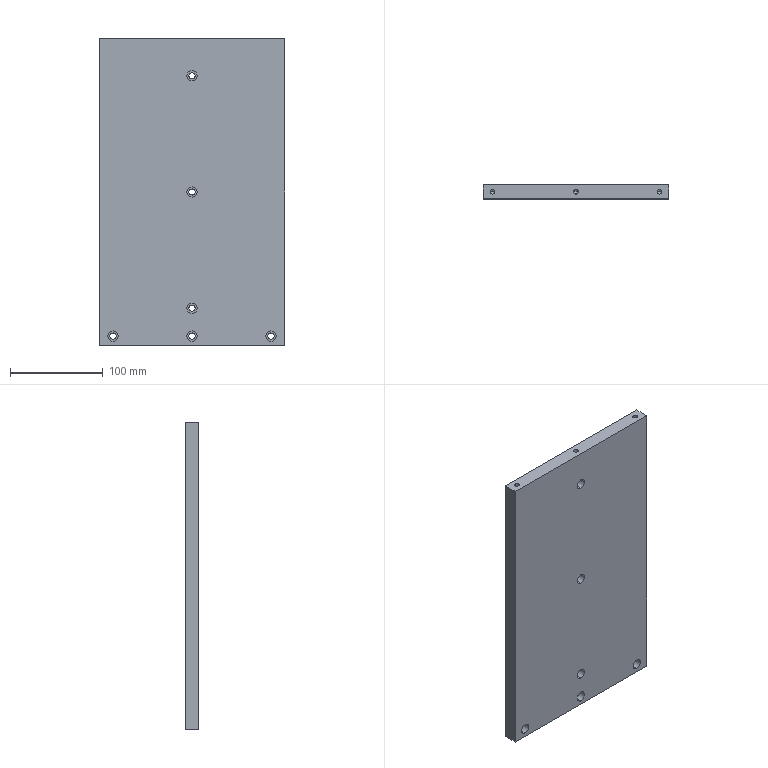Part | SolidWorks | features HoleWzd 3, Extrusion 1 | 1 solid | 48 faces | box 200 x 15 x 330 mm | volume 982971 mm3 | cylinder 30 | plane 12 | cone 6 | commonest cylinder face diameters 6.6 x12 11 x12 5 x6
STEP:
#1=CARTESIAN_POINT('',(-2.5,0.,148.));
#2=VERTEX_POINT('',#1);
#3=CARTESIAN_POINT('',(2.5,0.,148.));
#4=VERTEX_POINT('',#3);
#5=CARTESIAN_POINT('',(0.,0.,148.));
#6=DIRECTION('',(0.,0.,1.));
#7=DIRECTION('',(1.,0.,0.));
#8=AXIS2_PLACEMENT_3D('',#5,#6,#7);
#9=CIRCLE('',#8,2.5);
#10=EDGE_CURVE('',#2,#4,#9,.T.);
#11=ORIENTED_EDGE('',*,*,#10,.F.);
#12=CARTESIAN_POINT('',(-2.5,0.,165.));
#13=VERTEX_POINT('',#12);
#14=CARTESIAN_POINT('',(-2.5,0.,165.));
#15=DIRECTION('',(0.,0.,1.));
#16=VECTOR('',#15,1000.);
#17=LINE('',#14,#16);
#18=EDGE_CURVE('',#2,#13,#17,.T.);
#19=ORIENTED_EDGE('',*,*,#18,.T.);
#20=CARTESIAN_POINT('',(2.5,0.,165.));
#21=VERTEX_POINT('',#20);
#22=CARTESIAN_POINT('',(0.,0.,165.));
#23=DIRECTION('',(0.,0.,1.));
#24=DIRECTION('',(1.,0.,0.));
#25=AXIS2_PLACEMENT_3D('',#22,#23,#24);
#26=CIRCLE('',#25,2.5);
#27=EDGE_CURVE('',#13,#21,#26,.T.);
#28=ORIENTED_EDGE('',*,*,#27,.T.);
#29=CARTESIAN_POINT('',(2.5,0.,165.));
#30=DIRECTION('',(0.,0.,1.));
#31=VECTOR('',#30,1000.);
#32=LINE('',#29,#31);
#33=EDGE_CURVE('',#4,#21,#32,.T.);
#34=ORIENTED_EDGE('',*,*,#33,.F.);
#35=EDGE_LOOP('',(#11,#19,#28,#34));
#36=FACE_OUTER_BOUND('',#35,.T.);
#37=CARTESIAN_POINT('',(0.,0.,165.));
#38=DIRECTION('',(0.,0.,1.));
#39=DIRECTION('',(1.,0.,0.));
#40=AXIS2_PLACEMENT_3D('',#37,#38,#39);
#41=CYLINDRICAL_SURFACE('',#40,2.5);
#42=ADVANCED_FACE('',(#36),#41,.F.);
#43=CARTESIAN_POINT('',(0.,0.,146.498));
#44=VERTEX_POINT('',#43);
#45=CARTESIAN_POINT('',(2.5,0.,148.));
#46=DIRECTION('',(0.8572,0.,0.515));
#47=VECTOR('',#46,1000.);
#48=LINE('',#45,#47);
#49=EDGE_CURVE('',#44,#4,#48,.T.);
#50=ORIENTED_EDGE('',*,*,#49,.F.);
#51=CARTESIAN_POINT('',(-2.5,0.,148.));
#52=DIRECTION('',(-0.8572,0.,0.515));
#53=VECTOR('',#52,1000.);
#54=LINE('',#51,#53);
#55=EDGE_CURVE('',#44,#2,#54,.T.);
#56=ORIENTED_EDGE('',*,*,#55,.T.);
#57=ORIENTED_EDGE('',*,*,#10,.T.);
#58=EDGE_LOOP('',(#50,#56,#57));
#59=FACE_OUTER_BOUND('',#58,.T.);
#60=CARTESIAN_POINT('',(0.,0.,148.));
#61=DIRECTION('',(0.,0.,1.));
#62=DIRECTION('',(1.,0.,0.));
#63=AXIS2_PLACEMENT_3D('',#60,#61,#62);
#64=CONICAL_SURFACE('',#63,2.5,1.03);
#65=ADVANCED_FACE('',(#59),#64,.F.);
#66=CARTESIAN_POINT('',(-92.5,0.,148.));
#67=VERTEX_POINT('',#66);
#68=CARTESIAN_POINT('',(-87.5,0.,148.));
#69=VERTEX_POINT('',#68);
#70=CARTESIAN_POINT('',(-90.,0.,148.));
#71=DIRECTION('',(0.,0.,1.));
#72=DIRECTION('',(1.,0.,0.));
#73=AXIS2_PLACEMENT_3D('',#70,#71,#72);
#74=CIRCLE('',#73,2.5);
#75=EDGE_CURVE('',#67,#69,#74,.T.);
#76=ORIENTED_EDGE('',*,*,#75,.F.);
#77=CARTESIAN_POINT('',(-92.5,0.,165.));
#78=VERTEX_POINT('',#77);
#79=CARTESIAN_POINT('',(-92.5,0.,165.));
#80=DIRECTION('',(0.,0.,1.));
#81=VECTOR('',#80,1000.);
#82=LINE('',#79,#81);
#83=EDGE_CURVE('',#67,#78,#82,.T.);
#84=ORIENTED_EDGE('',*,*,#83,.T.);
#85=CARTESIAN_POINT('',(-87.5,0.,165.));
#86=VERTEX_POINT('',#85);
#87=CARTESIAN_POINT('',(-90.,0.,165.));
#88=DIRECTION('',(0.,0.,1.));
#89=DIRECTION('',(1.,0.,0.));
#90=AXIS2_PLACEMENT_3D('',#87,#88,#89);
#91=CIRCLE('',#90,2.5);
#92=EDGE_CURVE('',#78,#86,#91,.T.);
#93=ORIENTED_EDGE('',*,*,#92,.T.);
#94=CARTESIAN_POINT('',(-87.5,0.,165.));
#95=DIRECTION('',(0.,0.,1.));
#96=VECTOR('',#95,1000.);
#97=LINE('',#94,#96);
#98=EDGE_CURVE('',#69,#86,#97,.T.);
#99=ORIENTED_EDGE('',*,*,#98,.F.);
#100=EDGE_LOOP('',(#76,#84,#93,#99));
#101=FACE_OUTER_BOUND('',#100,.T.);
#102=CARTESIAN_POINT('',(-90.,0.,165.));
#103=DIRECTION('',(0.,0.,1.));
#104=DIRECTION('',(1.,0.,0.));
#105=AXIS2_PLACEMENT_3D('',#102,#103,#104);
#106=CYLINDRICAL_SURFACE('',#105,2.5);
#107=ADVANCED_FACE('',(#101),#106,.F.);
#108=CARTESIAN_POINT('',(-90.,0.,146.498));
#109=VERTEX_POINT('',#108);
#110=CARTESIAN_POINT('',(-87.5,0.,148.));
#111=DIRECTION('',(0.8572,0.,0.515));
#112=VECTOR('',#111,1000.);
#113=LINE('',#110,#112);
#114=EDGE_CURVE('',#109,#69,#113,.T.);
#115=ORIENTED_EDGE('',*,*,#114,.F.);
#116=CARTESIAN_POINT('',(-92.5,0.,148.));
#117=DIRECTION('',(-0.8572,0.,0.515));
#118=VECTOR('',#117,1000.);
#119=LINE('',#116,#118);
#120=EDGE_CURVE('',#109,#67,#119,.T.);
#121=ORIENTED_EDGE('',*,*,#120,.T.);
#122=ORIENTED_EDGE('',*,*,#75,.T.);
#123=EDGE_LOOP('',(#115,#121,#122));
#124=FACE_OUTER_BOUND('',#123,.T.);
#125=CARTESIAN_POINT('',(-90.,0.,148.));
#126=DIRECTION('',(0.,0.,1.));
#127=DIRECTION('',(1.,0.,0.));
#128=AXIS2_PLACEMENT_3D('',#125,#126,#127);
#129=CONICAL_SURFACE('',#128,2.5,1.03);
#130=ADVANCED_FACE('',(#124),#129,.F.);
#131=CARTESIAN_POINT('',(87.5,0.,148.));
#132=VERTEX_POINT('',#131);
#133=CARTESIAN_POINT('',(92.5,0.,148.));
#134=VERTEX_POINT('',#133);
#135=CARTESIAN_POINT('',(90.,0.,148.));
#136=DIRECTION('',(0.,0.,1.));
#137=DIRECTION('',(1.,0.,0.));
#138=AXIS2_PLACEMENT_3D('',#135,#136,#137);
#139=CIRCLE('',#138,2.5);
#140=EDGE_CURVE('',#132,#134,#139,.T.);
#141=ORIENTED_EDGE('',*,*,#140,.F.);
#142=CARTESIAN_POINT('',(87.5,0.,165.));
#143=VERTEX_POINT('',#142);
#144=CARTESIAN_POINT('',(87.5,0.,165.));
#145=DIRECTION('',(0.,0.,1.));
#146=VECTOR('',#145,1000.);
#147=LINE('',#144,#146);
#148=EDGE_CURVE('',#132,#143,#147,.T.);
#149=ORIENTED_EDGE('',*,*,#148,.T.);
#150=CARTESIAN_POINT('',(92.5,0.,165.));
#151=VERTEX_POINT('',#150);
#152=CARTESIAN_POINT('',(90.,0.,165.));
#153=DIRECTION('',(0.,0.,1.));
#154=DIRECTION('',(1.,0.,0.));
#155=AXIS2_PLACEMENT_3D('',#152,#153,#154);
#156=CIRCLE('',#155,2.5);
#157=EDGE_CURVE('',#143,#151,#156,.T.);
#158=ORIENTED_EDGE('',*,*,#157,.T.);
#159=CARTESIAN_POINT('',(92.5,0.,165.));
#160=DIRECTION('',(0.,0.,1.));
#161=VECTOR('',#160,1000.);
#162=LINE('',#159,#161);
#163=EDGE_CURVE('',#134,#151,#162,.T.);
#164=ORIENTED_EDGE('',*,*,#163,.F.);
#165=EDGE_LOOP('',(#141,#149,#158,#164));
#166=FACE_OUTER_BOUND('',#165,.T.);
#167=CARTESIAN_POINT('',(90.,0.,165.));
#168=DIRECTION('',(0.,0.,1.));
#169=DIRECTION('',(1.,0.,0.));
#170=AXIS2_PLACEMENT_3D('',#167,#168,#169);
#171=CYLINDRICAL_SURFACE('',#170,2.5);
#172=ADVANCED_FACE('',(#166),#171,.F.);
#173=CARTESIAN_POINT('',(90.,0.,146.498));
#174=VERTEX_POINT('',#173);
#175=CARTESIAN_POINT('',(92.5,0.,148.));
#176=DIRECTION('',(0.8572,0.,0.515));
#177=VECTOR('',#176,1000.);
#178=LINE('',#175,#177);
#179=EDGE_CURVE('',#174,#134,#178,.T.);
#180=ORIENTED_EDGE('',*,*,#179,.F.);
#181=CARTESIAN_POINT('',(87.5,0.,148.));
#182=DIRECTION('',(-0.8572,0.,0.515));
#183=VECTOR('',#182,1000.);
#184=LINE('',#181,#183);
#185=EDGE_CURVE('',#174,#132,#184,.T.);
#186=ORIENTED_EDGE('',*,*,#185,.T.);
#187=ORIENTED_EDGE('',*,*,#140,.T.);
#188=EDGE_LOOP('',(#180,#186,#187));
#189=FACE_OUTER_BOUND('',#188,.T.);
#190=CARTESIAN_POINT('',(90.,0.,148.));
#191=DIRECTION('',(0.,0.,1.));
#192=DIRECTION('',(1.,0.,0.));
#193=AXIS2_PLACEMENT_3D('',#190,#191,#192);
#194=CONICAL_SURFACE('',#193,2.5,1.03);
#195=ADVANCED_FACE('',(#189),#194,.F.);
#196=CARTESIAN_POINT('',(-85.,0.5,-149.5));
#197=VERTEX_POINT('',#196);
#198=CARTESIAN_POINT('',(-85.,0.5,-160.5));
#199=VERTEX_POINT('',#198);
#200=CARTESIAN_POINT('',(-85.,0.5,-155.));
#201=DIRECTION('',(0.,-1.,0.));
#202=DIRECTION('',(0.,0.,-1.));
#203=AXIS2_PLACEMENT_3D('',#200,#201,#202);
#204=CIRCLE('',#203,5.5);
#205=EDGE_CURVE('',#197,#199,#204,.T.);
#206=ORIENTED_EDGE('',*,*,#205,.F.);
#207=CARTESIAN_POINT('',(-85.,-7.5,-149.5));
#208=VERTEX_POINT('',#207);
#209=CARTESIAN_POINT('',(-85.,-7.5,-149.5));
#210=DIRECTION('',(0.,-1.,0.));
#211=VECTOR('',#210,1000.);
#212=LINE('',#209,#211);
#213=EDGE_CURVE('',#197,#208,#212,.T.);
#214=ORIENTED_EDGE('',*,*,#213,.T.);
#215=CARTESIAN_POINT('',(-85.,-7.5,-160.5));
#216=VERTEX_POINT('',#215);
#217=CARTESIAN_POINT('',(-85.,-7.5,-155.));
#218=DIRECTION('',(0.,-1.,0.));
#219=DIRECTION('',(0.,0.,-1.));
#220=AXIS2_PLACEMENT_3D('',#217,#218,#219);
#221=CIRCLE('',#220,5.5);
#222=EDGE_CURVE('',#208,#216,#221,.T.);
#223=ORIENTED_EDGE('',*,*,#222,.T.);
#224=CARTESIAN_POINT('',(-85.,-7.5,-160.5));
#225=DIRECTION('',(0.,-1.,0.));
#226=VECTOR('',#225,1000.);
#227=LINE('',#224,#226);
#228=EDGE_CURVE('',#199,#216,#227,.T.);
#229=ORIENTED_EDGE('',*,*,#228,.F.);
#230=EDGE_LOOP('',(#206,#214,#223,#229));
#231=FACE_OUTER_BOUND('',#230,.T.);
#232=CARTESIAN_POINT('',(-85.,-7.5,-155.));
#233=DIRECTION('',(0.,-1.,0.));
#234=DIRECTION('',(0.,0.,-1.));
#235=AXIS2_PLACEMENT_3D('',#232,#233,#234);
#236=CYLINDRICAL_SURFACE('',#235,5.5);
#237=ADVANCED_FACE('',(#231),#236,.F.);
#238=CARTESIAN_POINT('',(-85.,7.5,-151.7));
#239=VERTEX_POINT('',#238);
#240=CARTESIAN_POINT('',(-85.,7.5,-158.3));
#241=VERTEX_POINT('',#240);
#242=CARTESIAN_POINT('',(-85.,7.5,-155.));
#243=DIRECTION('',(0.,-1.,0.));
#244=DIRECTION('',(0.,0.,-1.));
#245=AXIS2_PLACEMENT_3D('',#242,#243,#244);
#246=CIRCLE('',#245,3.3);
#247=EDGE_CURVE('',#239,#241,#246,.T.);
#248=ORIENTED_EDGE('',*,*,#247,.F.);
#249=CARTESIAN_POINT('',(-85.,0.5,-151.7));
#250=VERTEX_POINT('',#249);
#251=CARTESIAN_POINT('',(-85.,-7.5,-151.7));
#252=DIRECTION('',(0.,-1.,0.));
#253=VECTOR('',#252,1000.);
#254=LINE('',#251,#253);
#255=EDGE_CURVE('',#239,#250,#254,.T.);
#256=ORIENTED_EDGE('',*,*,#255,.T.);
#257=CARTESIAN_POINT('',(-85.,0.5,-158.3));
#258=VERTEX_POINT('',#257);
#259=CARTESIAN_POINT('',(-85.,0.5,-155.));
#260=DIRECTION('',(0.,-1.,0.));
#261=DIRECTION('',(0.,0.,-1.));
#262=AXIS2_PLACEMENT_3D('',#259,#260,#261);
#263=CIRCLE('',#262,3.3);
#264=EDGE_CURVE('',#250,#258,#263,.T.);
#265=ORIENTED_EDGE('',*,*,#264,.T.);
#266=CARTESIAN_POINT('',(-85.,-7.5,-158.3));
#267=DIRECTION('',(0.,-1.,0.));
#268=VECTOR('',#267,1000.);
#269=LINE('',#266,#268);
#270=EDGE_CURVE('',#241,#258,#269,.T.);
#271=ORIENTED_EDGE('',*,*,#270,.F.);
#272=EDGE_LOOP('',(#248,#256,#265,#271));
#273=FACE_OUTER_BOUND('',#272,.T.);
#274=CARTESIAN_POINT('',(-85.,-7.5,-155.));
#275=DIRECTION('',(0.,-1.,0.));
#276=DIRECTION('',(0.,0.,-1.));
#277=AXIS2_PLACEMENT_3D('',#274,#275,#276);
#278=CYLINDRICAL_SURFACE('',#277,3.3);
#279=ADVANCED_FACE('',(#273),#278,.F.);
#280=CARTESIAN_POINT('',(0.,0.5,-149.5));
#281=VERTEX_POINT('',#280);
#282=CARTESIAN_POINT('',(0.,0.5,-160.5));
#283=VERTEX_POINT('',#282);
#284=CARTESIAN_POINT('',(0.,0.5,-155.));
#285=DIRECTION('',(0.,-1.,0.));
#286=DIRECTION('',(0.,0.,-1.));
#287=AXIS2_PLACEMENT_3D('',#284,#285,#286);
#288=CIRCLE('',#287,5.5);
#289=EDGE_CURVE('',#281,#283,#288,.T.);
#290=ORIENTED_EDGE('',*,*,#289,.F.);
#291=CARTESIAN_POINT('',(0.,-7.5,-149.5));
#292=VERTEX_POINT('',#291);
#293=CARTESIAN_POINT('',(0.,-7.5,-149.5));
#294=DIRECTION('',(0.,-1.,0.));
#295=VECTOR('',#294,1000.);
#296=LINE('',#293,#295);
#297=EDGE_CURVE('',#281,#292,#296,.T.);
#298=ORIENTED_EDGE('',*,*,#297,.T.);
#299=CARTESIAN_POINT('',(0.,-7.5,-160.5));
#300=VERTEX_POINT('',#299);
#301=CARTESIAN_POINT('',(0.,-7.5,-155.));
#302=DIRECTION('',(0.,-1.,0.));
#303=DIRECTION('',(0.,0.,-1.));
#304=AXIS2_PLACEMENT_3D('',#301,#302,#303);
#305=CIRCLE('',#304,5.5);
#306=EDGE_CURVE('',#292,#300,#305,.T.);
#307=ORIENTED_EDGE('',*,*,#306,.T.);
#308=CARTESIAN_POINT('',(0.,-7.5,-160.5));
#309=DIRECTION('',(0.,-1.,0.));
#310=VECTOR('',#309,1000.);
#311=LINE('',#308,#310);
#312=EDGE_CURVE('',#283,#300,#311,.T.);
#313=ORIENTED_EDGE('',*,*,#312,.F.);
#314=EDGE_LOOP('',(#290,#298,#307,#313));
#315=FACE_OUTER_BOUND('',#314,.T.);
#316=CARTESIAN_POINT('',(0.,-7.5,-155.));
#317=DIRECTION('',(0.,-1.,0.));
#318=DIRECTION('',(0.,0.,-1.));
#319=AXIS2_PLACEMENT_3D('',#316,#317,#318);
#320=CYLINDRICAL_SURFACE('',#319,5.5);
#321=ADVANCED_FACE('',(#315),#320,.F.);
#322=CARTESIAN_POINT('',(0.,7.5,-151.7));
#323=VERTEX_POINT('',#322);
#324=CARTESIAN_POINT('',(0.,7.5,-158.3));
#325=VERTEX_POINT('',#324);
#326=CARTESIAN_POINT('',(0.,7.5,-155.));
#327=DIRECTION('',(0.,-1.,0.));
#328=DIRECTION('',(0.,0.,-1.));
#329=AXIS2_PLACEMENT_3D('',#326,#327,#328);
#330=CIRCLE('',#329,3.3);
#331=EDGE_CURVE('',#323,#325,#330,.T.);
#332=ORIENTED_EDGE('',*,*,#331,.F.);
#333=CARTESIAN_POINT('',(0.,0.5,-151.7));
#334=VERTEX_POINT('',#333);
#335=CARTESIAN_POINT('',(0.,-7.5,-151.7));
#336=DIRECTION('',(0.,-1.,0.));
#337=VECTOR('',#336,1000.);
#338=LINE('',#335,#337);
#339=EDGE_CURVE('',#323,#334,#338,.T.);
#340=ORIENTED_EDGE('',*,*,#339,.T.);
#341=CARTESIAN_POINT('',(0.,0.5,-158.3));
#342=VERTEX_POINT('',#341);
#343=CARTESIAN_POINT('',(0.,0.5,-155.));
#344=DIRECTION('',(0.,-1.,0.));
#345=DIRECTION('',(0.,0.,-1.));
#346=AXIS2_PLACEMENT_3D('',#343,#344,#345);
#347=CIRCLE('',#346,3.3);
#348=EDGE_CURVE('',#334,#342,#347,.T.);
#349=ORIENTED_EDGE('',*,*,#348,.T.);
#350=CARTESIAN_POINT('',(0.,-7.5,-158.3));
#351=DIRECTION('',(0.,-1.,0.));
#352=VECTOR('',#351,1000.);
#353=LINE('',#350,#352);
#354=EDGE_CURVE('',#325,#342,#353,.T.);
#355=ORIENTED_EDGE('',*,*,#354,.F.);
#356=EDGE_LOOP('',(#332,#340,#349,#355));
#357=FACE_OUTER_BOUND('',#356,.T.);
#358=CARTESIAN_POINT('',(0.,-7.5,-155.));
#359=DIRECTION('',(0.,-1.,0.));
#360=DIRECTION('',(0.,0.,-1.));
#361=AXIS2_PLACEMENT_3D('',#358,#359,#360);
#362=CYLINDRICAL_SURFACE('',#361,3.3);
#363=ADVANCED_FACE('',(#357),#362,.F.);
#364=CARTESIAN_POINT('',(85.,0.5,-149.5));
#365=VERTEX_POINT('',#364);
#366=CARTESIAN_POINT('',(85.,0.5,-160.5));
#367=VERTEX_POINT('',#366);
#368=CARTESIAN_POINT('',(85.,0.5,-155.));
#369=DIRECTION('',(0.,-1.,0.));
#370=DIRECTION('',(0.,0.,-1.));
#371=AXIS2_PLACEMENT_3D('',#368,#369,#370);
#372=CIRCLE('',#371,5.5);
#373=EDGE_CURVE('',#365,#367,#372,.T.);
#374=ORIENTED_EDGE('',*,*,#373,.F.);
#375=CARTESIAN_POINT('',(85.,-7.5,-149.5));
#376=VERTEX_POINT('',#375);
#377=CARTESIAN_POINT('',(85.,-7.5,-149.5));
#378=DIRECTION('',(0.,-1.,0.));
#379=VECTOR('',#378,1000.);
#380=LINE('',#377,#379);
#381=EDGE_CURVE('',#365,#376,#380,.T.);
#382=ORIENTED_EDGE('',*,*,#381,.T.);
#383=CARTESIAN_POINT('',(85.,-7.5,-160.5));
#384=VERTEX_POINT('',#383);
#385=CARTESIAN_POINT('',(85.,-7.5,-155.));
#386=DIRECTION('',(0.,-1.,0.));
#387=DIRECTION('',(0.,0.,-1.));
#388=AXIS2_PLACEMENT_3D('',#385,#386,#387);
#389=CIRCLE('',#388,5.5);
#390=EDGE_CURVE('',#376,#384,#389,.T.);
#391=ORIENTED_EDGE('',*,*,#390,.T.);
#392=CARTESIAN_POINT('',(85.,-7.5,-160.5));
#393=DIRECTION('',(0.,-1.,0.));
#394=VECTOR('',#393,1000.);
#395=LINE('',#392,#394);
#396=EDGE_CURVE('',#367,#384,#395,.T.);
#397=ORIENTED_EDGE('',*,*,#396,.F.);
#398=EDGE_LOOP('',(#374,#382,#391,#397));
#399=FACE_OUTER_BOUND('',#398,.T.);
#400=CARTESIAN_POINT('',(85.,-7.5,-155.));
#401=DIRECTION('',(0.,-1.,0.));
#402=DIRECTION('',(0.,0.,-1.));
#403=AXIS2_PLACEMENT_3D('',#400,#401,#402);
#404=CYLINDRICAL_SURFACE('',#403,5.5);
#405=ADVANCED_FACE('',(#399),#404,.F.);
#406=CARTESIAN_POINT('',(85.,7.5,-151.7));
#407=VERTEX_POINT('',#406);
#408=CARTESIAN_POINT('',(85.,7.5,-158.3));
#409=VERTEX_POINT('',#408);
#410=CARTESIAN_POINT('',(85.,7.5,-155.));
#411=DIRECTION('',(0.,-1.,0.));
#412=DIRECTION('',(0.,0.,-1.));
#413=AXIS2_PLACEMENT_3D('',#410,#411,#412);
#414=CIRCLE('',#413,3.3);
#415=EDGE_CURVE('',#407,#409,#414,.T.);
#416=ORIENTED_EDGE('',*,*,#415,.F.);
#417=CARTESIAN_POINT('',(85.,0.5,-151.7));
#418=VERTEX_POINT('',#417);
#419=CARTESIAN_POINT('',(85.,-7.5,-151.7));
#420=DIRECTION('',(0.,-1.,0.));
#421=VECTOR('',#420,1000.);
#422=LINE('',#419,#421);
#423=EDGE_CURVE('',#407,#418,#422,.T.);
#424=ORIENTED_EDGE('',*,*,#423,.T.);
#425=CARTESIAN_POINT('',(85.,0.5,-158.3));
#426=VERTEX_POINT('',#425);
#427=CARTESIAN_POINT('',(85.,0.5,-155.));
#428=DIRECTION('',(0.,-1.,0.));
#429=DIRECTION('',(0.,0.,-1.));
#430=AXIS2_PLACEMENT_3D('',#427,#428,#429);
#431=CIRCLE('',#430,3.3);
#432=EDGE_CURVE('',#418,#426,#431,.T.);
#433=ORIENTED_EDGE('',*,*,#432,.T.);
#434=CARTESIAN_POINT('',(85.,-7.5,-158.3));
#435=DIRECTION('',(0.,-1.,0.));
#436=VECTOR('',#435,1000.);
#437=LINE('',#434,#436);
#438=EDGE_CURVE('',#409,#426,#437,.T.);
#439=ORIENTED_EDGE('',*,*,#438,.F.);
#440=EDGE_LOOP('',(#416,#424,#433,#439));
#441=FACE_OUTER_BOUND('',#440,.T.);
#442=CARTESIAN_POINT('',(85.,-7.5,-155.));
#443=DIRECTION('',(0.,-1.,0.));
#444=DIRECTION('',(0.,0.,-1.));
#445=AXIS2_PLACEMENT_3D('',#442,#443,#444);
#446=CYLINDRICAL_SURFACE('',#445,3.3);
#447=ADVANCED_FACE('',(#441),#446,.F.);
#448=CARTESIAN_POINT('',(0.,0.5,5.5));
#449=VERTEX_POINT('',#448);
#450=CARTESIAN_POINT('',(0.,0.5,-5.5));
#451=VERTEX_POINT('',#450);
#452=CARTESIAN_POINT('',(0.,0.5,0.));
#453=DIRECTION('',(0.,-1.,0.));
#454=DIRECTION('',(0.,0.,-1.));
#455=AXIS2_PLACEMENT_3D('',#452,#453,#454);
#456=CIRCLE('',#455,5.5);
#457=EDGE_CURVE('',#449,#451,#456,.T.);
#458=ORIENTED_EDGE('',*,*,#457,.F.);
#459=CARTESIAN_POINT('',(0.,-7.5,5.5));
#460=VERTEX_POINT('',#459);
#461=CARTESIAN_POINT('',(0.,-7.5,5.5));
#462=DIRECTION('',(0.,-1.,0.));
#463=VECTOR('',#462,1000.);
#464=LINE('',#461,#463);
#465=EDGE_CURVE('',#449,#460,#464,.T.);
#466=ORIENTED_EDGE('',*,*,#465,.T.);
#467=CARTESIAN_POINT('',(0.,-7.5,-5.5));
#468=VERTEX_POINT('',#467);
#469=CARTESIAN_POINT('',(0.,-7.5,0.));
#470=DIRECTION('',(0.,-1.,0.));
#471=DIRECTION('',(0.,0.,-1.));
#472=AXIS2_PLACEMENT_3D('',#469,#470,#471);
#473=CIRCLE('',#472,5.5);
#474=EDGE_CURVE('',#460,#468,#473,.T.);
#475=ORIENTED_EDGE('',*,*,#474,.T.);
#476=CARTESIAN_POINT('',(0.,-7.5,-5.5));
#477=DIRECTION('',(0.,-1.,0.));
#478=VECTOR('',#477,1000.);
#479=LINE('',#476,#478);
#480=EDGE_CURVE('',#451,#468,#479,.T.);
#481=ORIENTED_EDGE('',*,*,#480,.F.);
#482=EDGE_LOOP('',(#458,#466,#475,#481));
#483=FACE_OUTER_BOUND('',#482,.T.);
#484=CARTESIAN_POINT('',(0.,-7.5,0.));
#485=DIRECTION('',(0.,-1.,0.));
#486=DIRECTION('',(0.,0.,-1.));
#487=AXIS2_PLACEMENT_3D('',#484,#485,#486);
#488=CYLINDRICAL_SURFACE('',#487,5.5);
#489=ADVANCED_FACE('',(#483),#488,.F.);
#490=CARTESIAN_POINT('',(0.,7.5,3.3));
#491=VERTEX_POINT('',#490);
#492=CARTESIAN_POINT('',(0.,7.5,-3.3));
#493=VERTEX_POINT('',#492);
#494=CARTESIAN_POINT('',(0.,7.5,0.));
#495=DIRECTION('',(0.,-1.,0.));
#496=DIRECTION('',(0.,0.,-1.));
#497=AXIS2_PLACEMENT_3D('',#494,#495,#496);
#498=CIRCLE('',#497,3.3);
#499=EDGE_CURVE('',#491,#493,#498,.T.);
#500=ORIENTED_EDGE('',*,*,#499,.F.);
#501=CARTESIAN_POINT('',(0.,0.5,3.3));
#502=VERTEX_POINT('',#501);
#503=CARTESIAN_POINT('',(0.,-7.5,3.3));
#504=DIRECTION('',(0.,-1.,0.));
#505=VECTOR('',#504,1000.);
#506=LINE('',#503,#505);
#507=EDGE_CURVE('',#491,#502,#506,.T.);
#508=ORIENTED_EDGE('',*,*,#507,.T.);
#509=CARTESIAN_POINT('',(0.,0.5,-3.3));
#510=VERTEX_POINT('',#509);
#511=CARTESIAN_POINT('',(0.,0.5,0.));
#512=DIRECTION('',(0.,-1.,0.));
#513=DIRECTION('',(0.,0.,-1.));
#514=AXIS2_PLACEMENT_3D('',#511,#512,#513);
#515=CIRCLE('',#514,3.3);
#516=EDGE_CURVE('',#502,#510,#515,.T.);
#517=ORIENTED_EDGE('',*,*,#516,.T.);
#518=CARTESIAN_POINT('',(0.,-7.5,-3.3));
#519=DIRECTION('',(0.,-1.,0.));
#520=VECTOR('',#519,1000.);
#521=LINE('',#518,#520);
#522=EDGE_CURVE('',#493,#510,#521,.T.);
#523=ORIENTED_EDGE('',*,*,#522,.F.);
#524=EDGE_LOOP('',(#500,#508,#517,#523));
#525=FACE_OUTER_BOUND('',#524,.T.);
#526=CARTESIAN_POINT('',(0.,-7.5,0.));
#527=DIRECTION('',(0.,-1.,0.));
#528=DIRECTION('',(0.,0.,-1.));
#529=AXIS2_PLACEMENT_3D('',#526,#527,#528);
#530=CYLINDRICAL_SURFACE('',#529,3.3);
#531=ADVANCED_FACE('',(#525),#530,.F.);
#532=CARTESIAN_POINT('',(0.,0.5,130.5));
#533=VERTEX_POINT('',#532);
#534=CARTESIAN_POINT('',(0.,0.5,119.5));
#535=VERTEX_POINT('',#534);
#536=CARTESIAN_POINT('',(0.,0.5,125.));
#537=DIRECTION('',(0.,-1.,0.));
#538=DIRECTION('',(0.,0.,-1.));
#539=AXIS2_PLACEMENT_3D('',#536,#537,#538);
#540=CIRCLE('',#539,5.5);
#541=EDGE_CURVE('',#533,#535,#540,.T.);
#542=ORIENTED_EDGE('',*,*,#541,.F.);
#543=CARTESIAN_POINT('',(0.,-7.5,130.5));
#544=VERTEX_POINT('',#543);
#545=CARTESIAN_POINT('',(0.,-7.5,130.5));
#546=DIRECTION('',(0.,-1.,0.));
#547=VECTOR('',#546,1000.);
#548=LINE('',#545,#547);
#549=EDGE_CURVE('',#533,#544,#548,.T.);
#550=ORIENTED_EDGE('',*,*,#549,.T.);
#551=CARTESIAN_POINT('',(0.,-7.5,119.5));
#552=VERTEX_POINT('',#551);
#553=CARTESIAN_POINT('',(0.,-7.5,125.));
#554=DIRECTION('',(0.,-1.,0.));
#555=DIRECTION('',(0.,0.,-1.));
#556=AXIS2_PLACEMENT_3D('',#553,#554,#555);
#557=CIRCLE('',#556,5.5);
#558=EDGE_CURVE('',#544,#552,#557,.T.);
#559=ORIENTED_EDGE('',*,*,#558,.T.);
#560=CARTESIAN_POINT('',(0.,-7.5,119.5));
#561=DIRECTION('',(0.,-1.,0.));
#562=VECTOR('',#561,1000.);
#563=LINE('',#560,#562);
#564=EDGE_CURVE('',#535,#552,#563,.T.);
#565=ORIENTED_EDGE('',*,*,#564,.F.);
#566=EDGE_LOOP('',(#542,#550,#559,#565));
#567=FACE_OUTER_BOUND('',#566,.T.);
#568=CARTESIAN_POINT('',(0.,-7.5,125.));
#569=DIRECTION('',(0.,-1.,0.));
#570=DIRECTION('',(0.,0.,-1.));
#571=AXIS2_PLACEMENT_3D('',#568,#569,#570);
#572=CYLINDRICAL_SURFACE('',#571,5.5);
#573=ADVANCED_FACE('',(#567),#572,.F.);
#574=CARTESIAN_POINT('',(0.,7.5,128.3));
#575=VERTEX_POINT('',#574);
#576=CARTESIAN_POINT('',(0.,7.5,121.7));
#577=VERTEX_POINT('',#576);
#578=CARTESIAN_POINT('',(0.,7.5,125.));
#579=DIRECTION('',(0.,-1.,0.));
#580=DIRECTION('',(0.,0.,-1.));
#581=AXIS2_PLACEMENT_3D('',#578,#579,#580);
#582=CIRCLE('',#581,3.3);
#583=EDGE_CURVE('',#575,#577,#582,.T.);
#584=ORIENTED_EDGE('',*,*,#583,.F.);
#585=CARTESIAN_POINT('',(0.,0.5,128.3));
#586=VERTEX_POINT('',#585);
#587=CARTESIAN_POINT('',(0.,-7.5,128.3));
#588=DIRECTION('',(0.,-1.,0.));
#589=VECTOR('',#588,1000.);
#590=LINE('',#587,#589);
#591=EDGE_CURVE('',#575,#586,#590,.T.);
#592=ORIENTED_EDGE('',*,*,#591,.T.);
#593=CARTESIAN_POINT('',(0.,0.5,121.7));
#594=VERTEX_POINT('',#593);
#595=CARTESIAN_POINT('',(0.,0.5,125.));
#596=DIRECTION('',(0.,-1.,0.));
#597=DIRECTION('',(0.,0.,-1.));
#598=AXIS2_PLACEMENT_3D('',#595,#596,#597);
#599=CIRCLE('',#598,3.3);
#600=EDGE_CURVE('',#586,#594,#599,.T.);
#601=ORIENTED_EDGE('',*,*,#600,.T.);
#602=CARTESIAN_POINT('',(0.,-7.5,121.7));
#603=DIRECTION('',(0.,-1.,0.));
#604=VECTOR('',#603,1000.);
#605=LINE('',#602,#604);
#606=EDGE_CURVE('',#577,#594,#605,.T.);
#607=ORIENTED_EDGE('',*,*,#606,.F.);
#608=EDGE_LOOP('',(#584,#592,#601,#607));
#609=FACE_OUTER_BOUND('',#608,.T.);
#610=CARTESIAN_POINT('',(0.,-7.5,125.));
#611=DIRECTION('',(0.,-1.,0.));
#612=DIRECTION('',(0.,0.,-1.));
#613=AXIS2_PLACEMENT_3D('',#610,#611,#612);
#614=CYLINDRICAL_SURFACE('',#613,3.3);
#615=ADVANCED_FACE('',(#609),#614,.F.);
#616=CARTESIAN_POINT('',(0.,0.5,-119.5));
#617=VERTEX_POINT('',#616);
#618=CARTESIAN_POINT('',(0.,0.5,-130.5));
#619=VERTEX_POINT('',#618);
#620=CARTESIAN_POINT('',(0.,0.5,-125.));
#621=DIRECTION('',(0.,-1.,0.));
#622=DIRECTION('',(0.,0.,-1.));
#623=AXIS2_PLACEMENT_3D('',#620,#621,#622);
#624=CIRCLE('',#623,5.5);
#625=EDGE_CURVE('',#617,#619,#624,.T.);
#626=ORIENTED_EDGE('',*,*,#625,.F.);
#627=CARTESIAN_POINT('',(0.,-7.5,-119.5));
#628=VERTEX_POINT('',#627);
#629=CARTESIAN_POINT('',(0.,-7.5,-119.5));
#630=DIRECTION('',(0.,-1.,0.));
#631=VECTOR('',#630,1000.);
#632=LINE('',#629,#631);
#633=EDGE_CURVE('',#617,#628,#632,.T.);
#634=ORIENTED_EDGE('',*,*,#633,.T.);
#635=CARTESIAN_POINT('',(0.,-7.5,-130.5));
#636=VERTEX_POINT('',#635);
#637=CARTESIAN_POINT('',(0.,-7.5,-125.));
#638=DIRECTION('',(0.,-1.,0.));
#639=DIRECTION('',(0.,0.,-1.));
#640=AXIS2_PLACEMENT_3D('',#637,#638,#639);
#641=CIRCLE('',#640,5.5);
#642=EDGE_CURVE('',#628,#636,#641,.T.);
#643=ORIENTED_EDGE('',*,*,#642,.T.);
#644=CARTESIAN_POINT('',(0.,-7.5,-130.5));
#645=DIRECTION('',(0.,-1.,0.));
#646=VECTOR('',#645,1000.);
#647=LINE('',#644,#646);
#648=EDGE_CURVE('',#619,#636,#647,.T.);
#649=ORIENTED_EDGE('',*,*,#648,.F.);
#650=EDGE_LOOP('',(#626,#634,#643,#649));
#651=FACE_OUTER_BOUND('',#650,.T.);
#652=CARTESIAN_POINT('',(0.,-7.5,-125.));
#653=DIRECTION('',(0.,-1.,0.));
#654=DIRECTION('',(0.,0.,-1.));
#655=AXIS2_PLACEMENT_3D('',#652,#653,#654);
#656=CYLINDRICAL_SURFACE('',#655,5.5);
#657=ADVANCED_FACE('',(#651),#656,.F.);
#658=CARTESIAN_POINT('',(0.,7.5,-121.7));
#659=VERTEX_POINT('',#658);
#660=CARTESIAN_POINT('',(0.,7.5,-128.3));
#661=VERTEX_POINT('',#660);
#662=CARTESIAN_POINT('',(0.,7.5,-125.));
#663=DIRECTION('',(0.,-1.,0.));
#664=DIRECTION('',(0.,0.,-1.));
#665=AXIS2_PLACEMENT_3D('',#662,#663,#664);
#666=CIRCLE('',#665,3.3);
#667=EDGE_CURVE('',#659,#661,#666,.T.);
#668=ORIENTED_EDGE('',*,*,#667,.F.);
#669=CARTESIAN_POINT('',(0.,0.5,-121.7));
#670=VERTEX_POINT('',#669);
#671=CARTESIAN_POINT('',(0.,-7.5,-121.7));
#672=DIRECTION('',(0.,-1.,0.));
#673=VECTOR('',#672,1000.);
#674=LINE('',#671,#673);
#675=EDGE_CURVE('',#659,#670,#674,.T.);
#676=ORIENTED_EDGE('',*,*,#675,.T.);
#677=CARTESIAN_POINT('',(0.,0.5,-128.3));
#678=VERTEX_POINT('',#677);
#679=CARTESIAN_POINT('',(0.,0.5,-125.));
#680=DIRECTION('',(0.,-1.,0.));
#681=DIRECTION('',(0.,0.,-1.));
#682=AXIS2_PLACEMENT_3D('',#679,#680,#681);
#683=CIRCLE('',#682,3.3);
#684=EDGE_CURVE('',#670,#678,#683,.T.);
#685=ORIENTED_EDGE('',*,*,#684,.T.);
#686=CARTESIAN_POINT('',(0.,-7.5,-128.3));
#687=DIRECTION('',(0.,-1.,0.));
#688=VECTOR('',#687,1000.);
#689=LINE('',#686,#688);
#690=EDGE_CURVE('',#661,#678,#689,.T.);
#691=ORIENTED_EDGE('',*,*,#690,.F.);
#692=EDGE_LOOP('',(#668,#676,#685,#691));
#693=FACE_OUTER_BOUND('',#692,.T.);
#694=CARTESIAN_POINT('',(0.,-7.5,-125.));
#695=DIRECTION('',(0.,-1.,0.));
#696=DIRECTION('',(0.,0.,-1.));
#697=AXIS2_PLACEMENT_3D('',#694,#695,#696);
#698=CYLINDRICAL_SURFACE('',#697,3.3);
#699=ADVANCED_FACE('',(#693),#698,.F.);
#700=CARTESIAN_POINT('',(-100.,-7.5,-165.));
#701=VERTEX_POINT('',#700);
#702=CARTESIAN_POINT('',(-100.,-7.5,165.));
#703=VERTEX_POINT('',#702);
#704=CARTESIAN_POINT('',(-100.,-7.5,165.));
#705=DIRECTION('',(0.,0.,1.));
#706=VECTOR('',#705,1000.);
#707=LINE('',#704,#706);
#708=EDGE_CURVE('',#701,#703,#707,.T.);
#709=ORIENTED_EDGE('',*,*,#708,.T.);
#710=CARTESIAN_POINT('',(-100.,7.5,165.));
#711=VERTEX_POINT('',#710);
#712=CARTESIAN_POINT('',(-100.,7.5,165.));
#713=DIRECTION('',(0.,-1.,0.));
#714=VECTOR('',#713,1000.);
#715=LINE('',#712,#714);
#716=EDGE_CURVE('',#711,#703,#715,.T.);
#717=ORIENTED_EDGE('',*,*,#716,.F.);
#718=CARTESIAN_POINT('',(-100.,7.5,-165.));
#719=VERTEX_POINT('',#718);
#720=CARTESIAN_POINT('',(-100.,7.5,165.));
#721=DIRECTION('',(0.,0.,1.));
#722=VECTOR('',#721,1000.);
#723=LINE('',#720,#722);
#724=EDGE_CURVE('',#719,#711,#723,.T.);
#725=ORIENTED_EDGE('',*,*,#724,.F.);
#726=CARTESIAN_POINT('',(-100.,7.5,-165.));
#727=DIRECTION('',(0.,-1.,0.));
#728=VECTOR('',#727,1000.);
#729=LINE('',#726,#728);
#730=EDGE_CURVE('',#719,#701,#729,.T.);
#731=ORIENTED_EDGE('',*,*,#730,.T.);
#732=EDGE_LOOP('',(#709,#717,#725,#731));
#733=FACE_OUTER_BOUND('',#732,.T.);
#734=CARTESIAN_POINT('',(-100.,7.5,165.));
#735=DIRECTION('',(1.,0.,0.));
#736=DIRECTION('',(0.,0.,-1.));
#737=AXIS2_PLACEMENT_3D('',#734,#735,#736);
#738=PLANE('',#737);
#739=ADVANCED_FACE('',(#733),#738,.F.);
#740=CARTESIAN_POINT('',(0.,0.,165.));
#741=DIRECTION('',(0.,0.,1.));
#742=DIRECTION('',(1.,0.,0.));
#743=AXIS2_PLACEMENT_3D('',#740,#741,#742);
#744=CIRCLE('',#743,2.5);
#745=EDGE_CURVE('',#21,#13,#744,.T.);
#746=ORIENTED_EDGE('',*,*,#745,.F.);
#747=ORIENTED_EDGE('',*,*,#27,.F.);
#748=EDGE_LOOP('',(#746,#747));
#749=FACE_BOUND('',#748,.T.);
#750=CARTESIAN_POINT('',(-90.,0.,165.));
#751=DIRECTION('',(0.,0.,1.));
#752=DIRECTION('',(1.,0.,0.));
#753=AXIS2_PLACEMENT_3D('',#750,#751,#752);
#754=CIRCLE('',#753,2.5);
#755=EDGE_CURVE('',#86,#78,#754,.T.);
#756=ORIENTED_EDGE('',*,*,#755,.F.);
#757=ORIENTED_EDGE('',*,*,#92,.F.);
#758=EDGE_LOOP('',(#756,#757));
#759=FACE_BOUND('',#758,.T.);
#760=CARTESIAN_POINT('',(90.,0.,165.));
#761=DIRECTION('',(0.,0.,1.));
#762=DIRECTION('',(1.,0.,0.));
#763=AXIS2_PLACEMENT_3D('',#760,#761,#762);
#764=CIRCLE('',#763,2.5);
#765=EDGE_CURVE('',#151,#143,#764,.T.);
#766=ORIENTED_EDGE('',*,*,#765,.F.);
#767=ORIENTED_EDGE('',*,*,#157,.F.);
#768=EDGE_LOOP('',(#766,#767));
#769=FACE_BOUND('',#768,.T.);
#770=CARTESIAN_POINT('',(100.,-7.5,165.));
#771=VERTEX_POINT('',#770);
#772=CARTESIAN_POINT('',(100.,-7.5,165.));
#773=DIRECTION('',(1.,0.,0.));
#774=VECTOR('',#773,1000.);
#775=LINE('',#772,#774);
#776=EDGE_CURVE('',#703,#771,#775,.T.);
#777=ORIENTED_EDGE('',*,*,#776,.T.);
#778=CARTESIAN_POINT('',(100.,7.5,165.));
#779=VERTEX_POINT('',#778);
#780=CARTESIAN_POINT('',(100.,7.5,165.));
#781=DIRECTION('',(0.,-1.,0.));
#782=VECTOR('',#781,1000.);
#783=LINE('',#780,#782);
#784=EDGE_CURVE('',#779,#771,#783,.T.);
#785=ORIENTED_EDGE('',*,*,#784,.F.);
#786=CARTESIAN_POINT('',(100.,7.5,165.));
#787=DIRECTION('',(1.,0.,0.));
#788=VECTOR('',#787,1000.);
#789=LINE('',#786,#788);
#790=EDGE_CURVE('',#711,#779,#789,.T.);
#791=ORIENTED_EDGE('',*,*,#790,.F.);
#792=ORIENTED_EDGE('',*,*,#716,.T.);
#793=EDGE_LOOP('',(#777,#785,#791,#792));
#794=FACE_OUTER_BOUND('',#793,.T.);
#795=CARTESIAN_POINT('',(100.,7.5,165.));
#796=DIRECTION('',(0.,0.,-1.));
#797=DIRECTION('',(-1.,0.,0.));
#798=AXIS2_PLACEMENT_3D('',#795,#796,#797);
#799=PLANE('',#798);
#800=ADVANCED_FACE('',(#749,#759,#769,#794),#799,.F.);
#801=CARTESIAN_POINT('',(100.,-7.5,-165.));
#802=VERTEX_POINT('',#801);
#803=CARTESIAN_POINT('',(100.,-7.5,165.));
#804=DIRECTION('',(0.,0.,-1.));
#805=VECTOR('',#804,1000.);
#806=LINE('',#803,#805);
#807=EDGE_CURVE('',#771,#802,#806,.T.);
#808=ORIENTED_EDGE('',*,*,#807,.T.);
#809=CARTESIAN_POINT('',(100.,7.5,-165.));
#810=VERTEX_POINT('',#809);
#811=CARTESIAN_POINT('',(100.,7.5,-165.));
#812=DIRECTION('',(0.,-1.,0.));
#813=VECTOR('',#812,1000.);
#814=LINE('',#811,#813);
#815=EDGE_CURVE('',#810,#802,#814,.T.);
#816=ORIENTED_EDGE('',*,*,#815,.F.);
#817=CARTESIAN_POINT('',(100.,7.5,165.));
#818=DIRECTION('',(0.,0.,-1.));
#819=VECTOR('',#818,1000.);
#820=LINE('',#817,#819);
#821=EDGE_CURVE('',#779,#810,#820,.T.);
#822=ORIENTED_EDGE('',*,*,#821,.F.);
#823=ORIENTED_EDGE('',*,*,#784,.T.);
#824=EDGE_LOOP('',(#808,#816,#822,#823));
#825=FACE_OUTER_BOUND('',#824,.T.);
#826=CARTESIAN_POINT('',(100.,7.5,165.));
#827=DIRECTION('',(-1.,0.,0.));
#828=DIRECTION('',(0.,0.,1.));
#829=AXIS2_PLACEMENT_3D('',#826,#827,#828);
#830=PLANE('',#829);
#831=ADVANCED_FACE('',(#825),#830,.F.);
#832=CARTESIAN_POINT('',(100.,-7.5,-165.));
#833=DIRECTION('',(-1.,0.,0.));
#834=VECTOR('',#833,1000.);
#835=LINE('',#832,#834);
#836=EDGE_CURVE('',#802,#701,#835,.T.);
#837=ORIENTED_EDGE('',*,*,#836,.T.);
#838=ORIENTED_EDGE('',*,*,#730,.F.);
#839=CARTESIAN_POINT('',(100.,7.5,-165.));
#840=DIRECTION('',(-1.,0.,0.));
#841=VECTOR('',#840,1000.);
#842=LINE('',#839,#841);
#843=EDGE_CURVE('',#810,#719,#842,.T.);
#844=ORIENTED_EDGE('',*,*,#843,.F.);
#845=ORIENTED_EDGE('',*,*,#815,.T.);
#846=EDGE_LOOP('',(#837,#838,#844,#845));
#847=FACE_OUTER_BOUND('',#846,.T.);
#848=CARTESIAN_POINT('',(100.,7.5,-165.));
#849=DIRECTION('',(0.,0.,1.));
#850=DIRECTION('',(1.,0.,0.));
#851=AXIS2_PLACEMENT_3D('',#848,#849,#850);
#852=PLANE('',#851);
#853=ADVANCED_FACE('',(#847),#852,.F.);
#854=CARTESIAN_POINT('',(-85.,7.5,-155.));
#855=DIRECTION('',(0.,-1.,0.));
#856=DIRECTION('',(0.,0.,-1.));
#857=AXIS2_PLACEMENT_3D('',#854,#855,#856);
#858=CIRCLE('',#857,3.3);
#859=EDGE_CURVE('',#241,#239,#858,.T.);
#860=ORIENTED_EDGE('',*,*,#859,.T.);
#861=ORIENTED_EDGE('',*,*,#247,.T.);
#862=EDGE_LOOP('',(#860,#861));
#863=FACE_BOUND('',#862,.T.);
#864=CARTESIAN_POINT('',(0.,7.5,-155.));
#865=DIRECTION('',(0.,-1.,0.));
#866=DIRECTION('',(0.,0.,-1.));
#867=AXIS2_PLACEMENT_3D('',#864,#865,#866);
#868=CIRCLE('',#867,3.3);
#869=EDGE_CURVE('',#325,#323,#868,.T.);
#870=ORIENTED_EDGE('',*,*,#869,.T.);
#871=ORIENTED_EDGE('',*,*,#331,.T.);
#872=EDGE_LOOP('',(#870,#871));
#873=FACE_BOUND('',#872,.T.);
#874=CARTESIAN_POINT('',(85.,7.5,-155.));
#875=DIRECTION('',(0.,-1.,0.));
#876=DIRECTION('',(0.,0.,-1.));
#877=AXIS2_PLACEMENT_3D('',#874,#875,#876);
#878=CIRCLE('',#877,3.3);
#879=EDGE_CURVE('',#409,#407,#878,.T.);
#880=ORIENTED_EDGE('',*,*,#879,.T.);
#881=ORIENTED_EDGE('',*,*,#415,.T.);
#882=EDGE_LOOP('',(#880,#881));
#883=FACE_BOUND('',#882,.T.);
#884=CARTESIAN_POINT('',(0.,7.5,0.));
#885=DIRECTION('',(0.,-1.,0.));
#886=DIRECTION('',(0.,0.,-1.));
#887=AXIS2_PLACEMENT_3D('',#884,#885,#886);
#888=CIRCLE('',#887,3.3);
#889=EDGE_CURVE('',#493,#491,#888,.T.);
#890=ORIENTED_EDGE('',*,*,#889,.T.);
#891=ORIENTED_EDGE('',*,*,#499,.T.);
#892=EDGE_LOOP('',(#890,#891));
#893=FACE_BOUND('',#892,.T.);
#894=CARTESIAN_POINT('',(0.,7.5,125.));
#895=DIRECTION('',(0.,-1.,0.));
#896=DIRECTION('',(0.,0.,-1.));
#897=AXIS2_PLACEMENT_3D('',#894,#895,#896);
#898=CIRCLE('',#897,3.3);
#899=EDGE_CURVE('',#577,#575,#898,.T.);
#900=ORIENTED_EDGE('',*,*,#899,.T.);
#901=ORIENTED_EDGE('',*,*,#583,.T.);
#902=EDGE_LOOP('',(#900,#901));
#903=FACE_BOUND('',#902,.T.);
#904=CARTESIAN_POINT('',(0.,7.5,-125.));
#905=DIRECTION('',(0.,-1.,0.));
#906=DIRECTION('',(0.,0.,-1.));
#907=AXIS2_PLACEMENT_3D('',#904,#905,#906);
#908=CIRCLE('',#907,3.3);
#909=EDGE_CURVE('',#661,#659,#908,.T.);
#910=ORIENTED_EDGE('',*,*,#909,.T.);
#911=ORIENTED_EDGE('',*,*,#667,.T.);
#912=EDGE_LOOP('',(#910,#911));
#913=FACE_BOUND('',#912,.T.);
#914=ORIENTED_EDGE('',*,*,#724,.T.);
#915=ORIENTED_EDGE('',*,*,#790,.T.);
#916=ORIENTED_EDGE('',*,*,#821,.T.);
#917=ORIENTED_EDGE('',*,*,#843,.T.);
#918=EDGE_LOOP('',(#914,#915,#916,#917));
#919=FACE_OUTER_BOUND('',#918,.T.);
#920=CARTESIAN_POINT('',(0.,7.5,0.));
#921=DIRECTION('',(0.,1.,0.));
#922=DIRECTION('',(0.,0.,1.));
#923=AXIS2_PLACEMENT_3D('',#920,#921,#922);
#924=PLANE('',#923);
#925=ADVANCED_FACE('',(#863,#873,#883,#893,#903,#913,#919),#924,.T.);
#926=CARTESIAN_POINT('',(-85.,-7.5,-155.));
#927=DIRECTION('',(0.,-1.,0.));
#928=DIRECTION('',(0.,0.,-1.));
#929=AXIS2_PLACEMENT_3D('',#926,#927,#928);
#930=CIRCLE('',#929,5.5);
#931=EDGE_CURVE('',#216,#208,#930,.T.);
#932=ORIENTED_EDGE('',*,*,#931,.F.);
#933=ORIENTED_EDGE('',*,*,#222,.F.);
#934=EDGE_LOOP('',(#932,#933));
#935=FACE_BOUND('',#934,.T.);
#936=CARTESIAN_POINT('',(0.,-7.5,-155.));
#937=DIRECTION('',(0.,-1.,0.));
#938=DIRECTION('',(0.,0.,-1.));
#939=AXIS2_PLACEMENT_3D('',#936,#937,#938);
#940=CIRCLE('',#939,5.5);
#941=EDGE_CURVE('',#300,#292,#940,.T.);
#942=ORIENTED_EDGE('',*,*,#941,.F.);
#943=ORIENTED_EDGE('',*,*,#306,.F.);
#944=EDGE_LOOP('',(#942,#943));
#945=FACE_BOUND('',#944,.T.);
#946=CARTESIAN_POINT('',(85.,-7.5,-155.));
#947=DIRECTION('',(0.,-1.,0.));
#948=DIRECTION('',(0.,0.,-1.));
#949=AXIS2_PLACEMENT_3D('',#946,#947,#948);
#950=CIRCLE('',#949,5.5);
#951=EDGE_CURVE('',#384,#376,#950,.T.);
#952=ORIENTED_EDGE('',*,*,#951,.F.);
#953=ORIENTED_EDGE('',*,*,#390,.F.);
#954=EDGE_LOOP('',(#952,#953));
#955=FACE_BOUND('',#954,.T.);
#956=CARTESIAN_POINT('',(0.,-7.5,0.));
#957=DIRECTION('',(0.,-1.,0.));
#958=DIRECTION('',(0.,0.,-1.));
#959=AXIS2_PLACEMENT_3D('',#956,#957,#958);
#960=CIRCLE('',#959,5.5);
#961=EDGE_CURVE('',#468,#460,#960,.T.);
#962=ORIENTED_EDGE('',*,*,#961,.F.);
#963=ORIENTED_EDGE('',*,*,#474,.F.);
#964=EDGE_LOOP('',(#962,#963));
#965=FACE_BOUND('',#964,.T.);
#966=CARTESIAN_POINT('',(0.,-7.5,125.));
#967=DIRECTION('',(0.,-1.,0.));
#968=DIRECTION('',(0.,0.,-1.));
#969=AXIS2_PLACEMENT_3D('',#966,#967,#968);
#970=CIRCLE('',#969,5.5);
#971=EDGE_CURVE('',#552,#544,#970,.T.);
#972=ORIENTED_EDGE('',*,*,#971,.F.);
#973=ORIENTED_EDGE('',*,*,#558,.F.);
#974=EDGE_LOOP('',(#972,#973));
#975=FACE_BOUND('',#974,.T.);
#976=CARTESIAN_POINT('',(0.,-7.5,-125.));
#977=DIRECTION('',(0.,-1.,0.));
#978=DIRECTION('',(0.,0.,-1.));
#979=AXIS2_PLACEMENT_3D('',#976,#977,#978);
#980=CIRCLE('',#979,5.5);
#981=EDGE_CURVE('',#636,#628,#980,.T.);
#982=ORIENTED_EDGE('',*,*,#981,.F.);
#983=ORIENTED_EDGE('',*,*,#642,.F.);
#984=EDGE_LOOP('',(#982,#983));
#985=FACE_BOUND('',#984,.T.);
#986=ORIENTED_EDGE('',*,*,#708,.F.);
#987=ORIENTED_EDGE('',*,*,#836,.F.);
#988=ORIENTED_EDGE('',*,*,#807,.F.);
#989=ORIENTED_EDGE('',*,*,#776,.F.);
#990=EDGE_LOOP('',(#986,#987,#988,#989));
#991=FACE_OUTER_BOUND('',#990,.T.);
#992=CARTESIAN_POINT('',(0.,-7.5,0.));
#993=DIRECTION('',(0.,1.,0.));
#994=DIRECTION('',(0.,0.,1.));
#995=AXIS2_PLACEMENT_3D('',#992,#993,#994);
#996=PLANE('',#995);
#997=ADVANCED_FACE('',(#935,#945,#955,#965,#975,#985,#991),#996,.F.);
#998=ORIENTED_EDGE('',*,*,#675,.F.);
#999=ORIENTED_EDGE('',*,*,#909,.F.);
#1000=ORIENTED_EDGE('',*,*,#690,.T.);
#1001=CARTESIAN_POINT('',(0.,0.5,-125.));
#1002=DIRECTION('',(0.,-1.,0.));
#1003=DIRECTION('',(0.,0.,-1.));
#1004=AXIS2_PLACEMENT_3D('',#1001,#1002,#1003);
#1005=CIRCLE('',#1004,3.3);
#1006=EDGE_CURVE('',#678,#670,#1005,.T.);
#1007=ORIENTED_EDGE('',*,*,#1006,.T.);
#1008=EDGE_LOOP('',(#998,#999,#1000,#1007));
#1009=FACE_OUTER_BOUND('',#1008,.T.);
#1010=CARTESIAN_POINT('',(0.,-7.5,-125.));
#1011=DIRECTION('',(0.,-1.,0.));
#1012=DIRECTION('',(0.,0.,-1.));
#1013=AXIS2_PLACEMENT_3D('',#1010,#1011,#1012);
#1014=CYLINDRICAL_SURFACE('',#1013,3.3);
#1015=ADVANCED_FACE('',(#1009),#1014,.F.);
#1016=ORIENTED_EDGE('',*,*,#1006,.F.);
#1017=ORIENTED_EDGE('',*,*,#684,.F.);
#1018=EDGE_LOOP('',(#1016,#1017));
#1019=FACE_BOUND('',#1018,.T.);
#1020=CARTESIAN_POINT('',(0.,0.5,-125.));
#1021=DIRECTION('',(0.,-1.,0.));
#1022=DIRECTION('',(0.,0.,-1.));
#1023=AXIS2_PLACEMENT_3D('',#1020,#1021,#1022);
#1024=CIRCLE('',#1023,5.5);
#1025=EDGE_CURVE('',#619,#617,#1024,.T.);
#1026=ORIENTED_EDGE('',*,*,#1025,.T.);
#1027=ORIENTED_EDGE('',*,*,#625,.T.);
#1028=EDGE_LOOP('',(#1026,#1027));
#1029=FACE_OUTER_BOUND('',#1028,.T.);
#1030=CARTESIAN_POINT('',(3.3,0.5,-125.));
#1031=DIRECTION('',(0.,1.,0.));
#1032=DIRECTION('',(0.,0.,1.));
#1033=AXIS2_PLACEMENT_3D('',#1030,#1031,#1032);
#1034=PLANE('',#1033);
#1035=ADVANCED_FACE('',(#1019,#1029),#1034,.F.);
#1036=ORIENTED_EDGE('',*,*,#633,.F.);
#1037=ORIENTED_EDGE('',*,*,#1025,.F.);
#1038=ORIENTED_EDGE('',*,*,#648,.T.);
#1039=ORIENTED_EDGE('',*,*,#981,.T.);
#1040=EDGE_LOOP('',(#1036,#1037,#1038,#1039));
#1041=FACE_OUTER_BOUND('',#1040,.T.);
#1042=CARTESIAN_POINT('',(0.,-7.5,-125.));
#1043=DIRECTION('',(0.,-1.,0.));
#1044=DIRECTION('',(0.,0.,-1.));
#1045=AXIS2_PLACEMENT_3D('',#1042,#1043,#1044);
#1046=CYLINDRICAL_SURFACE('',#1045,5.5);
#1047=ADVANCED_FACE('',(#1041),#1046,.F.);
#1048=ORIENTED_EDGE('',*,*,#591,.F.);
#1049=ORIENTED_EDGE('',*,*,#899,.F.);
#1050=ORIENTED_EDGE('',*,*,#606,.T.);
#1051=CARTESIAN_POINT('',(0.,0.5,125.));
#1052=DIRECTION('',(0.,-1.,0.));
#1053=DIRECTION('',(0.,0.,-1.));
#1054=AXIS2_PLACEMENT_3D('',#1051,#1052,#1053);
#1055=CIRCLE('',#1054,3.3);
#1056=EDGE_CURVE('',#594,#586,#1055,.T.);
#1057=ORIENTED_EDGE('',*,*,#1056,.T.);
#1058=EDGE_LOOP('',(#1048,#1049,#1050,#1057));
#1059=FACE_OUTER_BOUND('',#1058,.T.);
#1060=CARTESIAN_POINT('',(0.,-7.5,125.));
#1061=DIRECTION('',(0.,-1.,0.));
#1062=DIRECTION('',(0.,0.,-1.));
#1063=AXIS2_PLACEMENT_3D('',#1060,#1061,#1062);
#1064=CYLINDRICAL_SURFACE('',#1063,3.3);
#1065=ADVANCED_FACE('',(#1059),#1064,.F.);
#1066=ORIENTED_EDGE('',*,*,#1056,.F.);
#1067=ORIENTED_EDGE('',*,*,#600,.F.);
#1068=EDGE_LOOP('',(#1066,#1067));
#1069=FACE_BOUND('',#1068,.T.);
#1070=CARTESIAN_POINT('',(0.,0.5,125.));
#1071=DIRECTION('',(0.,-1.,0.));
#1072=DIRECTION('',(0.,0.,-1.));
#1073=AXIS2_PLACEMENT_3D('',#1070,#1071,#1072);
#1074=CIRCLE('',#1073,5.5);
#1075=EDGE_CURVE('',#535,#533,#1074,.T.);
#1076=ORIENTED_EDGE('',*,*,#1075,.T.);
#1077=ORIENTED_EDGE('',*,*,#541,.T.);
#1078=EDGE_LOOP('',(#1076,#1077));
#1079=FACE_OUTER_BOUND('',#1078,.T.);
#1080=CARTESIAN_POINT('',(3.3,0.5,125.));
#1081=DIRECTION('',(0.,1.,0.));
#1082=DIRECTION('',(0.,0.,1.));
#1083=AXIS2_PLACEMENT_3D('',#1080,#1081,#1082);
#1084=PLANE('',#1083);
#1085=ADVANCED_FACE('',(#1069,#1079),#1084,.F.);
#1086=ORIENTED_EDGE('',*,*,#549,.F.);
#1087=ORIENTED_EDGE('',*,*,#1075,.F.);
#1088=ORIENTED_EDGE('',*,*,#564,.T.);
#1089=ORIENTED_EDGE('',*,*,#971,.T.);
#1090=EDGE_LOOP('',(#1086,#1087,#1088,#1089));
#1091=FACE_OUTER_BOUND('',#1090,.T.);
#1092=CARTESIAN_POINT('',(0.,-7.5,125.));
#1093=DIRECTION('',(0.,-1.,0.));
#1094=DIRECTION('',(0.,0.,-1.));
#1095=AXIS2_PLACEMENT_3D('',#1092,#1093,#1094);
#1096=CYLINDRICAL_SURFACE('',#1095,5.5);
#1097=ADVANCED_FACE('',(#1091),#1096,.F.);
#1098=ORIENTED_EDGE('',*,*,#507,.F.);
#1099=ORIENTED_EDGE('',*,*,#889,.F.);
#1100=ORIENTED_EDGE('',*,*,#522,.T.);
#1101=CARTESIAN_POINT('',(0.,0.5,0.));
#1102=DIRECTION('',(0.,-1.,0.));
#1103=DIRECTION('',(0.,0.,-1.));
#1104=AXIS2_PLACEMENT_3D('',#1101,#1102,#1103);
#1105=CIRCLE('',#1104,3.3);
#1106=EDGE_CURVE('',#510,#502,#1105,.T.);
#1107=ORIENTED_EDGE('',*,*,#1106,.T.);
#1108=EDGE_LOOP('',(#1098,#1099,#1100,#1107));
#1109=FACE_OUTER_BOUND('',#1108,.T.);
#1110=CARTESIAN_POINT('',(0.,-7.5,0.));
#1111=DIRECTION('',(0.,-1.,0.));
#1112=DIRECTION('',(0.,0.,-1.));
#1113=AXIS2_PLACEMENT_3D('',#1110,#1111,#1112);
#1114=CYLINDRICAL_SURFACE('',#1113,3.3);
#1115=ADVANCED_FACE('',(#1109),#1114,.F.);
#1116=ORIENTED_EDGE('',*,*,#1106,.F.);
#1117=ORIENTED_EDGE('',*,*,#516,.F.);
#1118=EDGE_LOOP('',(#1116,#1117));
#1119=FACE_BOUND('',#1118,.T.);
#1120=CARTESIAN_POINT('',(0.,0.5,0.));
#1121=DIRECTION('',(0.,-1.,0.));
#1122=DIRECTION('',(0.,0.,-1.));
#1123=AXIS2_PLACEMENT_3D('',#1120,#1121,#1122);
#1124=CIRCLE('',#1123,5.5);
#1125=EDGE_CURVE('',#451,#449,#1124,.T.);
#1126=ORIENTED_EDGE('',*,*,#1125,.T.);
#1127=ORIENTED_EDGE('',*,*,#457,.T.);
#1128=EDGE_LOOP('',(#1126,#1127));
#1129=FACE_OUTER_BOUND('',#1128,.T.);
#1130=CARTESIAN_POINT('',(3.3,0.5,0.));
#1131=DIRECTION('',(0.,1.,0.));
#1132=DIRECTION('',(0.,0.,1.));
#1133=AXIS2_PLACEMENT_3D('',#1130,#1131,#1132);
#1134=PLANE('',#1133);
#1135=ADVANCED_FACE('',(#1119,#1129),#1134,.F.);
#1136=ORIENTED_EDGE('',*,*,#465,.F.);
#1137=ORIENTED_EDGE('',*,*,#1125,.F.);
#1138=ORIENTED_EDGE('',*,*,#480,.T.);
#1139=ORIENTED_EDGE('',*,*,#961,.T.);
#1140=EDGE_LOOP('',(#1136,#1137,#1138,#1139));
#1141=FACE_OUTER_BOUND('',#1140,.T.);
#1142=CARTESIAN_POINT('',(0.,-7.5,0.));
#1143=DIRECTION('',(0.,-1.,0.));
#1144=DIRECTION('',(0.,0.,-1.));
#1145=AXIS2_PLACEMENT_3D('',#1142,#1143,#1144);
#1146=CYLINDRICAL_SURFACE('',#1145,5.5);
#1147=ADVANCED_FACE('',(#1141),#1146,.F.);
#1148=ORIENTED_EDGE('',*,*,#423,.F.);
#1149=ORIENTED_EDGE('',*,*,#879,.F.);
#1150=ORIENTED_EDGE('',*,*,#438,.T.);
#1151=CARTESIAN_POINT('',(85.,0.5,-155.));
#1152=DIRECTION('',(0.,-1.,0.));
#1153=DIRECTION('',(0.,0.,-1.));
#1154=AXIS2_PLACEMENT_3D('',#1151,#1152,#1153);
#1155=CIRCLE('',#1154,3.3);
#1156=EDGE_CURVE('',#426,#418,#1155,.T.);
#1157=ORIENTED_EDGE('',*,*,#1156,.T.);
#1158=EDGE_LOOP('',(#1148,#1149,#1150,#1157));
#1159=FACE_OUTER_BOUND('',#1158,.T.);
#1160=CARTESIAN_POINT('',(85.,-7.5,-155.));
#1161=DIRECTION('',(0.,-1.,0.));
#1162=DIRECTION('',(0.,0.,-1.));
#1163=AXIS2_PLACEMENT_3D('',#1160,#1161,#1162);
#1164=CYLINDRICAL_SURFACE('',#1163,3.3);
#1165=ADVANCED_FACE('',(#1159),#1164,.F.);
#1166=ORIENTED_EDGE('',*,*,#1156,.F.);
#1167=ORIENTED_EDGE('',*,*,#432,.F.);
#1168=EDGE_LOOP('',(#1166,#1167));
#1169=FACE_BOUND('',#1168,.T.);
#1170=CARTESIAN_POINT('',(85.,0.5,-155.));
#1171=DIRECTION('',(0.,-1.,0.));
#1172=DIRECTION('',(0.,0.,-1.));
#1173=AXIS2_PLACEMENT_3D('',#1170,#1171,#1172);
#1174=CIRCLE('',#1173,5.5);
#1175=EDGE_CURVE('',#367,#365,#1174,.T.);
#1176=ORIENTED_EDGE('',*,*,#1175,.T.);
#1177=ORIENTED_EDGE('',*,*,#373,.T.);
#1178=EDGE_LOOP('',(#1176,#1177));
#1179=FACE_OUTER_BOUND('',#1178,.T.);
#1180=CARTESIAN_POINT('',(88.3,0.5,-155.));
#1181=DIRECTION('',(0.,1.,0.));
#1182=DIRECTION('',(0.,0.,1.));
#1183=AXIS2_PLACEMENT_3D('',#1180,#1181,#1182);
#1184=PLANE('',#1183);
#1185=ADVANCED_FACE('',(#1169,#1179),#1184,.F.);
#1186=ORIENTED_EDGE('',*,*,#381,.F.);
#1187=ORIENTED_EDGE('',*,*,#1175,.F.);
#1188=ORIENTED_EDGE('',*,*,#396,.T.);
#1189=ORIENTED_EDGE('',*,*,#951,.T.);
#1190=EDGE_LOOP('',(#1186,#1187,#1188,#1189));
#1191=FACE_OUTER_BOUND('',#1190,.T.);
#1192=CARTESIAN_POINT('',(85.,-7.5,-155.));
#1193=DIRECTION('',(0.,-1.,0.));
#1194=DIRECTION('',(0.,0.,-1.));
#1195=AXIS2_PLACEMENT_3D('',#1192,#1193,#1194);
#1196=CYLINDRICAL_SURFACE('',#1195,5.5);
#1197=ADVANCED_FACE('',(#1191),#1196,.F.);
#1198=ORIENTED_EDGE('',*,*,#339,.F.);
#1199=ORIENTED_EDGE('',*,*,#869,.F.);
#1200=ORIENTED_EDGE('',*,*,#354,.T.);
#1201=CARTESIAN_POINT('',(0.,0.5,-155.));
#1202=DIRECTION('',(0.,-1.,0.));
#1203=DIRECTION('',(0.,0.,-1.));
#1204=AXIS2_PLACEMENT_3D('',#1201,#1202,#1203);
#1205=CIRCLE('',#1204,3.3);
#1206=EDGE_CURVE('',#342,#334,#1205,.T.);
#1207=ORIENTED_EDGE('',*,*,#1206,.T.);
#1208=EDGE_LOOP('',(#1198,#1199,#1200,#1207));
#1209=FACE_OUTER_BOUND('',#1208,.T.);
#1210=CARTESIAN_POINT('',(0.,-7.5,-155.));
#1211=DIRECTION('',(0.,-1.,0.));
#1212=DIRECTION('',(0.,0.,-1.));
#1213=AXIS2_PLACEMENT_3D('',#1210,#1211,#1212);
#1214=CYLINDRICAL_SURFACE('',#1213,3.3);
#1215=ADVANCED_FACE('',(#1209),#1214,.F.);
#1216=ORIENTED_EDGE('',*,*,#1206,.F.);
#1217=ORIENTED_EDGE('',*,*,#348,.F.);
#1218=EDGE_LOOP('',(#1216,#1217));
#1219=FACE_BOUND('',#1218,.T.);
#1220=CARTESIAN_POINT('',(0.,0.5,-155.));
#1221=DIRECTION('',(0.,-1.,0.));
#1222=DIRECTION('',(0.,0.,-1.));
#1223=AXIS2_PLACEMENT_3D('',#1220,#1221,#1222);
#1224=CIRCLE('',#1223,5.5);
#1225=EDGE_CURVE('',#283,#281,#1224,.T.);
#1226=ORIENTED_EDGE('',*,*,#1225,.T.);
#1227=ORIENTED_EDGE('',*,*,#289,.T.);
#1228=EDGE_LOOP('',(#1226,#1227));
#1229=FACE_OUTER_BOUND('',#1228,.T.);
#1230=CARTESIAN_POINT('',(3.3,0.5,-155.));
#1231=DIRECTION('',(0.,1.,0.));
#1232=DIRECTION('',(0.,0.,1.));
#1233=AXIS2_PLACEMENT_3D('',#1230,#1231,#1232);
#1234=PLANE('',#1233);
#1235=ADVANCED_FACE('',(#1219,#1229),#1234,.F.);
#1236=ORIENTED_EDGE('',*,*,#297,.F.);
#1237=ORIENTED_EDGE('',*,*,#1225,.F.);
#1238=ORIENTED_EDGE('',*,*,#312,.T.);
#1239=ORIENTED_EDGE('',*,*,#941,.T.);
#1240=EDGE_LOOP('',(#1236,#1237,#1238,#1239));
#1241=FACE_OUTER_BOUND('',#1240,.T.);
#1242=CARTESIAN_POINT('',(0.,-7.5,-155.));
#1243=DIRECTION('',(0.,-1.,0.));
#1244=DIRECTION('',(0.,0.,-1.));
#1245=AXIS2_PLACEMENT_3D('',#1242,#1243,#1244);
#1246=CYLINDRICAL_SURFACE('',#1245,5.5);
#1247=ADVANCED_FACE('',(#1241),#1246,.F.);
#1248=ORIENTED_EDGE('',*,*,#255,.F.);
#1249=ORIENTED_EDGE('',*,*,#859,.F.);
#1250=ORIENTED_EDGE('',*,*,#270,.T.);
#1251=CARTESIAN_POINT('',(-85.,0.5,-155.));
#1252=DIRECTION('',(0.,-1.,0.));
#1253=DIRECTION('',(0.,0.,-1.));
#1254=AXIS2_PLACEMENT_3D('',#1251,#1252,#1253);
#1255=CIRCLE('',#1254,3.3);
#1256=EDGE_CURVE('',#258,#250,#1255,.T.);
#1257=ORIENTED_EDGE('',*,*,#1256,.T.);
#1258=EDGE_LOOP('',(#1248,#1249,#1250,#1257));
#1259=FACE_OUTER_BOUND('',#1258,.T.);
#1260=CARTESIAN_POINT('',(-85.,-7.5,-155.));
#1261=DIRECTION('',(0.,-1.,0.));
#1262=DIRECTION('',(0.,0.,-1.));
#1263=AXIS2_PLACEMENT_3D('',#1260,#1261,#1262);
#1264=CYLINDRICAL_SURFACE('',#1263,3.3);
#1265=ADVANCED_FACE('',(#1259),#1264,.F.);
#1266=ORIENTED_EDGE('',*,*,#1256,.F.);
#1267=ORIENTED_EDGE('',*,*,#264,.F.);
#1268=EDGE_LOOP('',(#1266,#1267));
#1269=FACE_BOUND('',#1268,.T.);
#1270=CARTESIAN_POINT('',(-85.,0.5,-155.));
#1271=DIRECTION('',(0.,-1.,0.));
#1272=DIRECTION('',(0.,0.,-1.));
#1273=AXIS2_PLACEMENT_3D('',#1270,#1271,#1272);
#1274=CIRCLE('',#1273,5.5);
#1275=EDGE_CURVE('',#199,#197,#1274,.T.);
#1276=ORIENTED_EDGE('',*,*,#1275,.T.);
#1277=ORIENTED_EDGE('',*,*,#205,.T.);
#1278=EDGE_LOOP('',(#1276,#1277));
#1279=FACE_OUTER_BOUND('',#1278,.T.);
#1280=CARTESIAN_POINT('',(-81.7,0.5,-155.));
#1281=DIRECTION('',(0.,1.,0.));
#1282=DIRECTION('',(0.,0.,1.));
#1283=AXIS2_PLACEMENT_3D('',#1280,#1281,#1282);
#1284=PLANE('',#1283);
#1285=ADVANCED_FACE('',(#1269,#1279),#1284,.F.);
#1286=ORIENTED_EDGE('',*,*,#213,.F.);
#1287=ORIENTED_EDGE('',*,*,#1275,.F.);
#1288=ORIENTED_EDGE('',*,*,#228,.T.);
#1289=ORIENTED_EDGE('',*,*,#931,.T.);
#1290=EDGE_LOOP('',(#1286,#1287,#1288,#1289));
#1291=FACE_OUTER_BOUND('',#1290,.T.);
#1292=CARTESIAN_POINT('',(-85.,-7.5,-155.));
#1293=DIRECTION('',(0.,-1.,0.));
#1294=DIRECTION('',(0.,0.,-1.));
#1295=AXIS2_PLACEMENT_3D('',#1292,#1293,#1294);
#1296=CYLINDRICAL_SURFACE('',#1295,5.5);
#1297=ADVANCED_FACE('',(#1291),#1296,.F.);
#1298=ORIENTED_EDGE('',*,*,#185,.F.);
#1299=ORIENTED_EDGE('',*,*,#179,.T.);
#1300=CARTESIAN_POINT('',(90.,0.,148.));
#1301=DIRECTION('',(0.,0.,1.));
#1302=DIRECTION('',(1.,0.,0.));
#1303=AXIS2_PLACEMENT_3D('',#1300,#1301,#1302);
#1304=CIRCLE('',#1303,2.5);
#1305=EDGE_CURVE('',#134,#132,#1304,.T.);
#1306=ORIENTED_EDGE('',*,*,#1305,.T.);
#1307=EDGE_LOOP('',(#1298,#1299,#1306));
#1308=FACE_OUTER_BOUND('',#1307,.T.);
#1309=CARTESIAN_POINT('',(90.,0.,148.));
#1310=DIRECTION('',(0.,0.,1.));
#1311=DIRECTION('',(1.,0.,0.));
#1312=AXIS2_PLACEMENT_3D('',#1309,#1310,#1311);
#1313=CONICAL_SURFACE('',#1312,2.5,1.03);
#1314=ADVANCED_FACE('',(#1308),#1313,.F.);
#1315=ORIENTED_EDGE('',*,*,#148,.F.);
#1316=ORIENTED_EDGE('',*,*,#1305,.F.);
#1317=ORIENTED_EDGE('',*,*,#163,.T.);
#1318=ORIENTED_EDGE('',*,*,#765,.T.);
#1319=EDGE_LOOP('',(#1315,#1316,#1317,#1318));
#1320=FACE_OUTER_BOUND('',#1319,.T.);
#1321=CARTESIAN_POINT('',(90.,0.,165.));
#1322=DIRECTION('',(0.,0.,1.));
#1323=DIRECTION('',(1.,0.,0.));
#1324=AXIS2_PLACEMENT_3D('',#1321,#1322,#1323);
#1325=CYLINDRICAL_SURFACE('',#1324,2.5);
#1326=ADVANCED_FACE('',(#1320),#1325,.F.);
#1327=ORIENTED_EDGE('',*,*,#120,.F.);
#1328=ORIENTED_EDGE('',*,*,#114,.T.);
#1329=CARTESIAN_POINT('',(-90.,0.,148.));
#1330=DIRECTION('',(0.,0.,1.));
#1331=DIRECTION('',(1.,0.,0.));
#1332=AXIS2_PLACEMENT_3D('',#1329,#1330,#1331);
#1333=CIRCLE('',#1332,2.5);
#1334=EDGE_CURVE('',#69,#67,#1333,.T.);
#1335=ORIENTED_EDGE('',*,*,#1334,.T.);
#1336=EDGE_LOOP('',(#1327,#1328,#1335));
#1337=FACE_OUTER_BOUND('',#1336,.T.);
#1338=CARTESIAN_POINT('',(-90.,0.,148.));
#1339=DIRECTION('',(0.,0.,1.));
#1340=DIRECTION('',(1.,0.,0.));
#1341=AXIS2_PLACEMENT_3D('',#1338,#1339,#1340);
#1342=CONICAL_SURFACE('',#1341,2.5,1.03);
#1343=ADVANCED_FACE('',(#1337),#1342,.F.);
#1344=ORIENTED_EDGE('',*,*,#83,.F.);
#1345=ORIENTED_EDGE('',*,*,#1334,.F.);
#1346=ORIENTED_EDGE('',*,*,#98,.T.);
#1347=ORIENTED_EDGE('',*,*,#755,.T.);
#1348=EDGE_LOOP('',(#1344,#1345,#1346,#1347));
#1349=FACE_OUTER_BOUND('',#1348,.T.);
#1350=CARTESIAN_POINT('',(-90.,0.,165.));
#1351=DIRECTION('',(0.,0.,1.));
#1352=DIRECTION('',(1.,0.,0.));
#1353=AXIS2_PLACEMENT_3D('',#1350,#1351,#1352);
#1354=CYLINDRICAL_SURFACE('',#1353,2.5);
#1355=ADVANCED_FACE('',(#1349),#1354,.F.);
#1356=ORIENTED_EDGE('',*,*,#55,.F.);
#1357=ORIENTED_EDGE('',*,*,#49,.T.);
#1358=CARTESIAN_POINT('',(0.,0.,148.));
#1359=DIRECTION('',(0.,0.,1.));
#1360=DIRECTION('',(1.,0.,0.));
#1361=AXIS2_PLACEMENT_3D('',#1358,#1359,#1360);
#1362=CIRCLE('',#1361,2.5);
#1363=EDGE_CURVE('',#4,#2,#1362,.T.);
#1364=ORIENTED_EDGE('',*,*,#1363,.T.);
#1365=EDGE_LOOP('',(#1356,#1357,#1364));
#1366=FACE_OUTER_BOUND('',#1365,.T.);
#1367=CARTESIAN_POINT('',(0.,0.,148.));
#1368=DIRECTION('',(0.,0.,1.));
#1369=DIRECTION('',(1.,0.,0.));
#1370=AXIS2_PLACEMENT_3D('',#1367,#1368,#1369);
#1371=CONICAL_SURFACE('',#1370,2.5,1.03);
#1372=ADVANCED_FACE('',(#1366),#1371,.F.);
#1373=ORIENTED_EDGE('',*,*,#18,.F.);
#1374=ORIENTED_EDGE('',*,*,#1363,.F.);
#1375=ORIENTED_EDGE('',*,*,#33,.T.);
#1376=ORIENTED_EDGE('',*,*,#745,.T.);
#1377=EDGE_LOOP('',(#1373,#1374,#1375,#1376));
#1378=FACE_OUTER_BOUND('',#1377,.T.);
#1379=CARTESIAN_POINT('',(0.,0.,165.));
#1380=DIRECTION('',(0.,0.,1.));
#1381=DIRECTION('',(1.,0.,0.));
#1382=AXIS2_PLACEMENT_3D('',#1379,#1380,#1381);
#1383=CYLINDRICAL_SURFACE('',#1382,2.5);
#1384=ADVANCED_FACE('',(#1378),#1383,.F.);
#1385=CLOSED_SHELL('',(#42,#65,#107,#130,#172,#195,#237,#279,#321,#363,#405,#447,#489,#531,#573,#615,#657,#699,#739,#800,#831,#853,#925,#997,#1015,#1035,#1047,#1065,#1085,#1097,#1115,#1135,#1147,#1165,#1185,#1197,#1215,#1235,#1247,#1265,#1285,#1297,#1314,#1326,#1343,#1355,#1372,#1384));
#1386=MANIFOLD_SOLID_BREP('',#1385);
#1387=CARTESIAN_POINT('',(0.,0.,0.));
#1388=DIRECTION('',(0.,0.,1.));
#1389=DIRECTION('',(1.,0.,0.));
#1390=AXIS2_PLACEMENT_3D('',#1387,#1388,#1389);
#1391=(LENGTH_UNIT()NAMED_UNIT(*)SI_UNIT(.MILLI.,.METRE.));
#1392=UNCERTAINTY_MEASURE_WITH_UNIT(LENGTH_MEASURE(0.00001),#1391,'','');
#1393=(NAMED_UNIT(*)PLANE_ANGLE_UNIT()SI_UNIT($,.RADIAN.));
#1394=(NAMED_UNIT(*)SI_UNIT($,.STERADIAN.)SOLID_ANGLE_UNIT());
#1395=(GEOMETRIC_REPRESENTATION_CONTEXT(3)GLOBAL_UNCERTAINTY_ASSIGNED_CONTEXT((#1392))GLOBAL_UNIT_ASSIGNED_CONTEXT((#1391,#1393,#1394))REPRESENTATION_CONTEXT('',''));
#1396=ADVANCED_BREP_SHAPE_REPRESENTATION('',(#1386,#1390),#1395);